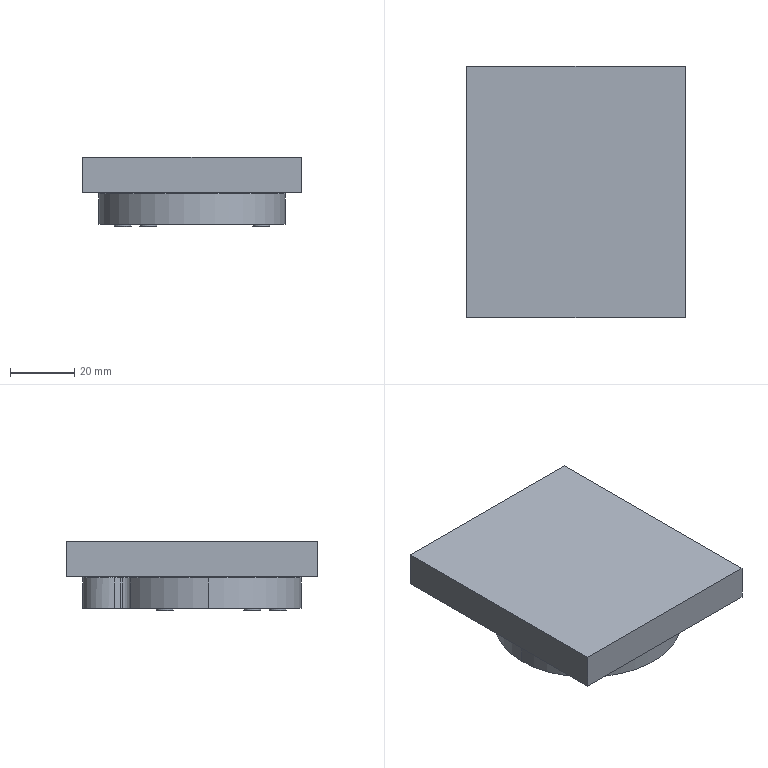NC program | NX | posted with a generic post | part box 68 x 78.27 x 21.8 mm
Lines 3280 to 3502 of 3502:
(SPOT_DRILLING , TOOL : D6A45)
N6522 T01 M6
N6524 G54
N6526 G17 G0 G90 X-21.562 Y8.479 S9500 M3
N6528 G43 Z30. H1
N6530 G94 G82 G98 Z-7. F250. P200 R-3.
N6532 X0. Y2.865 Z-1. R3.
N6534 Y-13.135
N6536 X-13.614 Y-26.697 Z-7. R-3.
N6538 X21.562 Y-18.748
N6540 G80
N6542 G0 X21.562 Y-18.748 Z30.
N6544 M5
(DRILLING_COPY_COPY_COPY , TOOL : 1.6ZT)
N6546 T16 M6
N6548 G54
N6550 G17 G0 G90 X0. Y2.865 S2500 M3
N6552 G43 Z30. H16
N6554 G94 G83 G98 Z-9.981 F80. Q2. R3.
N6556 Y-13.135
N6558 G80
N6560 G0 X0. Y-13.135 Z30.
N6562 M5
(DRILLING_COPY_COPY_COPY_1 , TOOL : 3.5ZT)
N6564 T07 M6
N6566 G54
N6568 G17 G0 G90 X-21.562 Y8.479 S2500 M3
N6570 G43 Z30. H7
N6572 G94 G83 G98 Z-19.352 F100. Q2. R-3.
N6574 X-13.614 Y-26.697
N6576 X21.562 Y-18.748
N6578 G80
N6580 G0 X21.562 Y-18.748 Z30.
N6582 M5
(HOLE_MILLING_2 , TOOL : D4)
N6584 T11 M6
N6586 G54
N6588 G17 G0 G90 X-21.562 Y8.479 S9500 M3
N6590 G43 Z30. H11
N6592 Z-5.5
N6594 G94 G3 X-21.062 Y7.979 R0.5 F1250.
N6596 X-20.562 Y8.479 R0.5
N6598 X-20.562 Y8.479 Z-5.9 I-1. J0.
N6600 X-20.562 Y8.479 Z-6.3 I-1. J0.
N6602 X-20.562 Y8.479 Z-6.7 I-1. J0.
N6604 X-20.562 Y8.479 Z-7.1 I-1. J0.
N6606 X-20.562 Y8.479 Z-7.5 I-1. J0.
N6608 X-20.562 Y8.479 Z-7.9 I-1. J0.
N6610 X-20.562 Y8.479 Z-8.3 I-1. J0.
N6612 X-20.562 Y8.479 Z-8.7 I-1. J0.
N6614 X-20.562 Y8.479 Z-9.1 I-1. J0.
N6616 X-20.562 Y8.479 Z-9.5 I-1. J0.
N6618 X-20.562 Y8.479 Z-9.9 I-1. J0.
N6620 X-20.562 Y8.479 Z-10.3 I-1. J0.
N6622 X-20.562 Y8.479 Z-10.7 I-1. J0.
N6624 X-20.562 Y8.479 Z-11.1 I-1. J0.
N6626 X-20.562 Y8.479 Z-11.5 I-1. J0.
N6628 X-20.562 Y8.479 Z-11.9 I-1. J0.
N6630 X-20.562 Y8.479 Z-12.3 I-1. J0.
N6632 X-20.562 Y8.479 Z-12.7 I-1. J0.
N6634 X-21.562 Y7.479 Z-13. R-1.
N6636 X-20.562 Y8.479 R1.
N6638 X-21.562 Y7.479 R-1.
N6640 X-21.062 Y7.979 R0.5
N6642 X-21.562 Y8.479 R0.5
N6644 G0 Z30.
N6646 X-13.614 Y-26.697
N6648 Z-5.5
N6650 G3 X-13.114 Y-27.197 R0.5
N6652 X-12.614 Y-26.697 R0.5
N6654 X-12.614 Y-26.697 Z-5.9 I-1. J0.
N6656 X-12.614 Y-26.697 Z-6.3 I-1. J0.
N6658 X-12.614 Y-26.697 Z-6.7 I-1. J0.
N6660 X-12.614 Y-26.697 Z-7.1 I-1. J0.
N6662 X-12.614 Y-26.697 Z-7.5 I-1. J0.
N6664 X-12.614 Y-26.697 Z-7.9 I-1. J0.
N6666 X-12.614 Y-26.697 Z-8.3 I-1. J0.
N6668 X-12.614 Y-26.697 Z-8.7 I-1. J0.
N6670 X-12.614 Y-26.697 Z-9.1 I-1. J0.
N6672 X-12.614 Y-26.697 Z-9.5 I-1. J0.
N6674 X-12.614 Y-26.697 Z-9.9 I-1. J0.
N6676 X-12.614 Y-26.697 Z-10.3 I-1. J0.
N6678 X-12.614 Y-26.697 Z-10.7 I-1. J0.
N6680 X-12.614 Y-26.697 Z-11.1 I-1. J0.
N6682 X-12.614 Y-26.697 Z-11.5 I-1. J0.
N6684 X-12.614 Y-26.697 Z-11.9 I-1. J0.
N6686 X-12.614 Y-26.697 Z-12.3 I-1. J0.
N6688 X-12.614 Y-26.697 Z-12.7 I-1. J0.
N6690 X-13.614 Y-27.697 Z-13. R-1.
N6692 X-12.614 Y-26.697 R1.
N6694 X-13.614 Y-27.697 R-1.
N6696 X-13.114 Y-27.197 R0.5
N6698 X-13.614 Y-26.697 R0.5
N6700 G0 Z30.
N6702 X21.562 Y-18.748
N6704 Z-5.5
N6706 G3 X22.062 Y-19.248 R0.5
N6708 X22.562 Y-18.748 R0.5
N6710 X22.562 Y-18.748 Z-5.9 I-1. J0.
N6712 X22.562 Y-18.748 Z-6.3 I-1. J0.
N6714 X22.562 Y-18.748 Z-6.7 I-1. J0.
N6716 X22.562 Y-18.748 Z-7.1 I-1. J0.
N6718 X22.562 Y-18.748 Z-7.5 I-1. J0.
N6720 X22.562 Y-18.748 Z-7.9 I-1. J0.
N6722 X22.562 Y-18.748 Z-8.3 I-1. J0.
N6724 X22.562 Y-18.748 Z-8.7 I-1. J0.
N6726 X22.562 Y-18.748 Z-9.1 I-1. J0.
N6728 X22.562 Y-18.748 Z-9.5 I-1. J0.
N6730 X22.562 Y-18.748 Z-9.9 I-1. J0.
N6732 X22.562 Y-18.748 Z-10.3 I-1. J0.
N6734 X22.562 Y-18.748 Z-10.7 I-1. J0.
N6736 X22.562 Y-18.748 Z-11.1 I-1. J0.
N6738 X22.562 Y-18.748 Z-11.5 I-1. J0.
N6740 X22.562 Y-18.748 Z-11.9 I-1. J0.
N6742 X22.562 Y-18.748 Z-12.3 I-1. J0.
N6744 X22.562 Y-18.748 Z-12.7 I-1. J0.
N6746 X21.562 Y-19.748 Z-13. R-1.
N6748 X22.562 Y-18.748 R1.
N6750 X21.562 Y-19.748 R-1.
N6752 X22.062 Y-19.248 R0.5
N6754 X21.562 Y-18.748 R0.5
N6756 G0 Z30.
N6758 M5
(PLANAR_PROFILE , TOOL : D6A45)
N6760 T01 M6
N6762 G54
N6764 G17 G0 G90 X-19.512 Y8.202 S9500 M3
N6766 G43 Z30. H1
N6768 Z-5.5
N6770 G94 G1 Y8.831 Z-5.669 F500.
N6772 X-19.866 Y9.683 Z-5.916
N6774 X-20.555 Y10.299 Z-6.163
N6776 X-21.442 Y10.555 Z-6.411
N6778 X-22.353 Y10.403 Z-6.658
N6780 X-23.107 Y9.871 Z-6.906
N6782 X-23.295 Y9.573 Z-7.
N6784 G3 X-22.656 Y6.745 R2.05 F1500.
N6786 X-23.295 Y9.573 R-2.05
N6788 G1 Z-5.5
N6790 G0 Z30.
N6792 X-27.417 Y5.6
N6794 Z-5.5
N6796 G1 X-27.155 Y6.34 Z-5.71 F500.
N6798 X-25.612 Y9.463 Z-6.644
N6800 X-24.902 Y10.588 Z-7.
N6802 G2 X-16.175 Y19.475 R29.45 F1500.
N6804 G3 X-15.089 Y22.168 R2.55
N6806 G1 X-15.495 Y23.967
N6808 G2 X-5.956 Y34.521 R8.7
N6810 X-4.944 Y34.16 R2.45
N6812 G1 X-0.426 Y31.307
N6814 G2 X0.335 Y30.549 R2.45
N6816 X1.477 Y27.802 R8.7
N6818 G1 X1.883 Y26.003
N6820 G3 X4.022 Y24.039 R2.55
N6822 G2 X-24.902 Y10.588 R-29.45
N6824 G1 Z-5.5
N6826 G0 Z30.
N6828 X-12.607 Y-26.996
N6830 Z-5.5
N6832 G1 Z-7. F500.
N6834 X-11.864 Y-27.216
N6836 G3 X-11.564 Y-26.697 R0.6
N6838 X-13.614 Y-24.647 R2.05 F1500.
N6840 X-11.564 Y-26.697 R-2.05
N6842 X-11.864 Y-26.177 R0.6
N6844 G1 X-12.607 Y-26.398
N6846 Z-5.5
N6848 G0 Z30.
N6850 X22.569 Y-19.047
N6852 Z-5.5
N6854 G1 Z-7. F500.
N6856 X23.312 Y-19.268
N6858 G3 X23.612 Y-18.748 R0.6
N6860 X21.562 Y-16.698 R2.05 F1500.
N6862 X23.612 Y-18.748 R-2.05
N6864 X23.312 Y-18.229 R0.6
N6866 G1 X22.569 Y-18.45
N6868 Z-5.5
N6870 G0 Z30.
(PLANAR_PROFILE_COPY , TOOL : D6A45)
N6872 X3.945 Y-9.605
N6874 Z0.5
N6876 G1 Z-1. F500.
N6878 X4.221 Y-10.364
N6880 G3 X4.804 Y-10.226 R0.6
N6882 X4.804 Y-0.044 R7. F1500.
N6884 X3.775 Y0.365 R1.5
N6886 G1 X-3.775
N6888 G3 X-4.804 Y-0.044 R1.5
N6890 X-4.804 Y-10.226 R7.
N6892 X-3.775 Y-10.635 R1.5
N6894 G1 X3.775
N6896 G3 X4.804 Y-10.226 R1.5
N6898 X4.976 Y-9.651 R0.6
N6900 G1 X4.769 Y-8.776
N6902 Z0.5
N6904 G0 Z30.
N6906 X11.464 Y-4.232
N6908 Z0.5
N6910 G1 Z-1. F500.
N6912 X10.8 Y-4.615
N6914 G3 X10.5 Y-5.135 R0.6
N6916 G2 X0. Y-15.635 R10.5 F1500.
N6918 X10.5 Y-5.135 R-10.5
N6920 G3 X10.8 Y-5.654 R0.6
N6922 G1 X11.464 Y-6.038
N6924 Z0.5
N6926 G0 Z30.
N6928 M5
N6930 M2